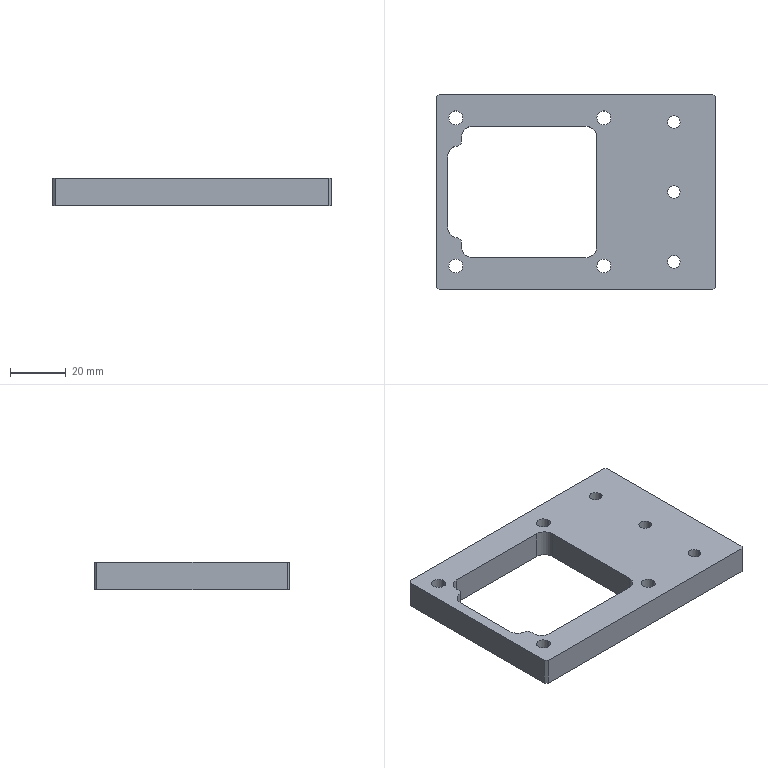Part | STEP file | MYT-A01-P13 | 1 solid | 47 faces | box 100 x 70 x 10 mm | volume 43994 mm3 | cylinder 26 | plane 21 | commonest cylinder face diameters 8 x12 5 x8 4.5 x6
STEP:
#1=CARTESIAN_POINT('',(39.,-25.,4.6));
#2=VERTEX_POINT('',#1);
#3=CARTESIAN_POINT('',(31.,-25.,4.6));
#4=VERTEX_POINT('',#3);
#5=CARTESIAN_POINT('',(35.,-25.,4.6));
#6=DIRECTION('',(0.,0.,-1.));
#7=DIRECTION('',(-1.,0.,0.));
#8=AXIS2_PLACEMENT_3D('',#5,#6,#7);
#9=CIRCLE('',#8,4.);
#10=EDGE_CURVE('',#2,#4,#9,.T.);
#11=ORIENTED_EDGE('',*,*,#10,.F.);
#12=CARTESIAN_POINT('',(39.,-25.,0.));
#13=VERTEX_POINT('',#12);
#14=CARTESIAN_POINT('',(39.,-25.,0.));
#15=DIRECTION('',(0.,0.,-1.));
#16=VECTOR('',#15,1000.);
#17=LINE('',#14,#16);
#18=EDGE_CURVE('',#2,#13,#17,.T.);
#19=ORIENTED_EDGE('',*,*,#18,.T.);
#20=CARTESIAN_POINT('',(31.,-25.,0.));
#21=VERTEX_POINT('',#20);
#22=CARTESIAN_POINT('',(35.,-25.,0.));
#23=DIRECTION('',(0.,0.,-1.));
#24=DIRECTION('',(-1.,0.,0.));
#25=AXIS2_PLACEMENT_3D('',#22,#23,#24);
#26=CIRCLE('',#25,4.);
#27=EDGE_CURVE('',#13,#21,#26,.T.);
#28=ORIENTED_EDGE('',*,*,#27,.T.);
#29=CARTESIAN_POINT('',(31.,-25.,0.));
#30=DIRECTION('',(0.,0.,-1.));
#31=VECTOR('',#30,1000.);
#32=LINE('',#29,#31);
#33=EDGE_CURVE('',#4,#21,#32,.T.);
#34=ORIENTED_EDGE('',*,*,#33,.F.);
#35=EDGE_LOOP('',(#11,#19,#28,#34));
#36=FACE_OUTER_BOUND('',#35,.T.);
#37=CARTESIAN_POINT('',(35.,-25.,0.));
#38=DIRECTION('',(0.,0.,-1.));
#39=DIRECTION('',(-1.,0.,0.));
#40=AXIS2_PLACEMENT_3D('',#37,#38,#39);
#41=CYLINDRICAL_SURFACE('',#40,4.);
#42=ADVANCED_FACE('',(#36),#41,.F.);
#43=CARTESIAN_POINT('',(37.25,-25.,10.));
#44=VERTEX_POINT('',#43);
#45=CARTESIAN_POINT('',(32.75,-25.,10.));
#46=VERTEX_POINT('',#45);
#47=CARTESIAN_POINT('',(35.,-25.,10.));
#48=DIRECTION('',(0.,0.,-1.));
#49=DIRECTION('',(-1.,0.,0.));
#50=AXIS2_PLACEMENT_3D('',#47,#48,#49);
#51=CIRCLE('',#50,2.25);
#52=EDGE_CURVE('',#44,#46,#51,.T.);
#53=ORIENTED_EDGE('',*,*,#52,.F.);
#54=CARTESIAN_POINT('',(37.25,-25.,4.6));
#55=VERTEX_POINT('',#54);
#56=CARTESIAN_POINT('',(37.25,-25.,0.));
#57=DIRECTION('',(0.,0.,-1.));
#58=VECTOR('',#57,1000.);
#59=LINE('',#56,#58);
#60=EDGE_CURVE('',#44,#55,#59,.T.);
#61=ORIENTED_EDGE('',*,*,#60,.T.);
#62=CARTESIAN_POINT('',(32.75,-25.,4.6));
#63=VERTEX_POINT('',#62);
#64=CARTESIAN_POINT('',(35.,-25.,4.6));
#65=DIRECTION('',(0.,0.,-1.));
#66=DIRECTION('',(-1.,0.,0.));
#67=AXIS2_PLACEMENT_3D('',#64,#65,#66);
#68=CIRCLE('',#67,2.25);
#69=EDGE_CURVE('',#55,#63,#68,.T.);
#70=ORIENTED_EDGE('',*,*,#69,.T.);
#71=CARTESIAN_POINT('',(32.75,-25.,0.));
#72=DIRECTION('',(0.,0.,-1.));
#73=VECTOR('',#72,1000.);
#74=LINE('',#71,#73);
#75=EDGE_CURVE('',#46,#63,#74,.T.);
#76=ORIENTED_EDGE('',*,*,#75,.F.);
#77=EDGE_LOOP('',(#53,#61,#70,#76));
#78=FACE_OUTER_BOUND('',#77,.T.);
#79=CARTESIAN_POINT('',(35.,-25.,0.));
#80=DIRECTION('',(0.,0.,-1.));
#81=DIRECTION('',(-1.,0.,0.));
#82=AXIS2_PLACEMENT_3D('',#79,#80,#81);
#83=CYLINDRICAL_SURFACE('',#82,2.25);
#84=ADVANCED_FACE('',(#78),#83,.F.);
#85=CARTESIAN_POINT('',(39.,0.,4.6));
#86=VERTEX_POINT('',#85);
#87=CARTESIAN_POINT('',(31.,0.,4.6));
#88=VERTEX_POINT('',#87);
#89=CARTESIAN_POINT('',(35.,0.,4.6));
#90=DIRECTION('',(0.,0.,-1.));
#91=DIRECTION('',(-1.,0.,0.));
#92=AXIS2_PLACEMENT_3D('',#89,#90,#91);
#93=CIRCLE('',#92,4.);
#94=EDGE_CURVE('',#86,#88,#93,.T.);
#95=ORIENTED_EDGE('',*,*,#94,.F.);
#96=CARTESIAN_POINT('',(39.,0.,0.));
#97=VERTEX_POINT('',#96);
#98=CARTESIAN_POINT('',(39.,0.,0.));
#99=DIRECTION('',(0.,0.,-1.));
#100=VECTOR('',#99,1000.);
#101=LINE('',#98,#100);
#102=EDGE_CURVE('',#86,#97,#101,.T.);
#103=ORIENTED_EDGE('',*,*,#102,.T.);
#104=CARTESIAN_POINT('',(31.,0.,0.));
#105=VERTEX_POINT('',#104);
#106=CARTESIAN_POINT('',(35.,0.,0.));
#107=DIRECTION('',(0.,0.,-1.));
#108=DIRECTION('',(-1.,0.,0.));
#109=AXIS2_PLACEMENT_3D('',#106,#107,#108);
#110=CIRCLE('',#109,4.);
#111=EDGE_CURVE('',#97,#105,#110,.T.);
#112=ORIENTED_EDGE('',*,*,#111,.T.);
#113=CARTESIAN_POINT('',(31.,0.,0.));
#114=DIRECTION('',(0.,0.,-1.));
#115=VECTOR('',#114,1000.);
#116=LINE('',#113,#115);
#117=EDGE_CURVE('',#88,#105,#116,.T.);
#118=ORIENTED_EDGE('',*,*,#117,.F.);
#119=EDGE_LOOP('',(#95,#103,#112,#118));
#120=FACE_OUTER_BOUND('',#119,.T.);
#121=CARTESIAN_POINT('',(35.,0.,0.));
#122=DIRECTION('',(0.,0.,-1.));
#123=DIRECTION('',(-1.,0.,0.));
#124=AXIS2_PLACEMENT_3D('',#121,#122,#123);
#125=CYLINDRICAL_SURFACE('',#124,4.);
#126=ADVANCED_FACE('',(#120),#125,.F.);
#127=CARTESIAN_POINT('',(37.25,0.,10.));
#128=VERTEX_POINT('',#127);
#129=CARTESIAN_POINT('',(32.75,0.,10.));
#130=VERTEX_POINT('',#129);
#131=CARTESIAN_POINT('',(35.,0.,10.));
#132=DIRECTION('',(0.,0.,-1.));
#133=DIRECTION('',(-1.,0.,0.));
#134=AXIS2_PLACEMENT_3D('',#131,#132,#133);
#135=CIRCLE('',#134,2.25);
#136=EDGE_CURVE('',#128,#130,#135,.T.);
#137=ORIENTED_EDGE('',*,*,#136,.F.);
#138=CARTESIAN_POINT('',(37.25,0.,4.6));
#139=VERTEX_POINT('',#138);
#140=CARTESIAN_POINT('',(37.25,0.,0.));
#141=DIRECTION('',(0.,0.,-1.));
#142=VECTOR('',#141,1000.);
#143=LINE('',#140,#142);
#144=EDGE_CURVE('',#128,#139,#143,.T.);
#145=ORIENTED_EDGE('',*,*,#144,.T.);
#146=CARTESIAN_POINT('',(32.75,0.,4.6));
#147=VERTEX_POINT('',#146);
#148=CARTESIAN_POINT('',(35.,0.,4.6));
#149=DIRECTION('',(0.,0.,-1.));
#150=DIRECTION('',(-1.,0.,0.));
#151=AXIS2_PLACEMENT_3D('',#148,#149,#150);
#152=CIRCLE('',#151,2.25);
#153=EDGE_CURVE('',#139,#147,#152,.T.);
#154=ORIENTED_EDGE('',*,*,#153,.T.);
#155=CARTESIAN_POINT('',(32.75,0.,0.));
#156=DIRECTION('',(0.,0.,-1.));
#157=VECTOR('',#156,1000.);
#158=LINE('',#155,#157);
#159=EDGE_CURVE('',#130,#147,#158,.T.);
#160=ORIENTED_EDGE('',*,*,#159,.F.);
#161=EDGE_LOOP('',(#137,#145,#154,#160));
#162=FACE_OUTER_BOUND('',#161,.T.);
#163=CARTESIAN_POINT('',(35.,0.,0.));
#164=DIRECTION('',(0.,0.,-1.));
#165=DIRECTION('',(-1.,0.,0.));
#166=AXIS2_PLACEMENT_3D('',#163,#164,#165);
#167=CYLINDRICAL_SURFACE('',#166,2.25);
#168=ADVANCED_FACE('',(#162),#167,.F.);
#169=CARTESIAN_POINT('',(39.,25.,4.6));
#170=VERTEX_POINT('',#169);
#171=CARTESIAN_POINT('',(31.,25.,4.6));
#172=VERTEX_POINT('',#171);
#173=CARTESIAN_POINT('',(35.,25.,4.6));
#174=DIRECTION('',(0.,0.,-1.));
#175=DIRECTION('',(-1.,0.,0.));
#176=AXIS2_PLACEMENT_3D('',#173,#174,#175);
#177=CIRCLE('',#176,4.);
#178=EDGE_CURVE('',#170,#172,#177,.T.);
#179=ORIENTED_EDGE('',*,*,#178,.F.);
#180=CARTESIAN_POINT('',(39.,25.,0.));
#181=VERTEX_POINT('',#180);
#182=CARTESIAN_POINT('',(39.,25.,0.));
#183=DIRECTION('',(0.,0.,-1.));
#184=VECTOR('',#183,1000.);
#185=LINE('',#182,#184);
#186=EDGE_CURVE('',#170,#181,#185,.T.);
#187=ORIENTED_EDGE('',*,*,#186,.T.);
#188=CARTESIAN_POINT('',(31.,25.,0.));
#189=VERTEX_POINT('',#188);
#190=CARTESIAN_POINT('',(35.,25.,0.));
#191=DIRECTION('',(0.,0.,-1.));
#192=DIRECTION('',(-1.,0.,0.));
#193=AXIS2_PLACEMENT_3D('',#190,#191,#192);
#194=CIRCLE('',#193,4.);
#195=EDGE_CURVE('',#181,#189,#194,.T.);
#196=ORIENTED_EDGE('',*,*,#195,.T.);
#197=CARTESIAN_POINT('',(31.,25.,0.));
#198=DIRECTION('',(0.,0.,-1.));
#199=VECTOR('',#198,1000.);
#200=LINE('',#197,#199);
#201=EDGE_CURVE('',#172,#189,#200,.T.);
#202=ORIENTED_EDGE('',*,*,#201,.F.);
#203=EDGE_LOOP('',(#179,#187,#196,#202));
#204=FACE_OUTER_BOUND('',#203,.T.);
#205=CARTESIAN_POINT('',(35.,25.,0.));
#206=DIRECTION('',(0.,0.,-1.));
#207=DIRECTION('',(-1.,0.,0.));
#208=AXIS2_PLACEMENT_3D('',#205,#206,#207);
#209=CYLINDRICAL_SURFACE('',#208,4.);
#210=ADVANCED_FACE('',(#204),#209,.F.);
#211=CARTESIAN_POINT('',(37.25,25.,10.));
#212=VERTEX_POINT('',#211);
#213=CARTESIAN_POINT('',(32.75,25.,10.));
#214=VERTEX_POINT('',#213);
#215=CARTESIAN_POINT('',(35.,25.,10.));
#216=DIRECTION('',(0.,0.,-1.));
#217=DIRECTION('',(-1.,0.,0.));
#218=AXIS2_PLACEMENT_3D('',#215,#216,#217);
#219=CIRCLE('',#218,2.25);
#220=EDGE_CURVE('',#212,#214,#219,.T.);
#221=ORIENTED_EDGE('',*,*,#220,.F.);
#222=CARTESIAN_POINT('',(37.25,25.,4.6));
#223=VERTEX_POINT('',#222);
#224=CARTESIAN_POINT('',(37.25,25.,0.));
#225=DIRECTION('',(0.,0.,-1.));
#226=VECTOR('',#225,1000.);
#227=LINE('',#224,#226);
#228=EDGE_CURVE('',#212,#223,#227,.T.);
#229=ORIENTED_EDGE('',*,*,#228,.T.);
#230=CARTESIAN_POINT('',(32.75,25.,4.6));
#231=VERTEX_POINT('',#230);
#232=CARTESIAN_POINT('',(35.,25.,4.6));
#233=DIRECTION('',(0.,0.,-1.));
#234=DIRECTION('',(-1.,0.,0.));
#235=AXIS2_PLACEMENT_3D('',#232,#233,#234);
#236=CIRCLE('',#235,2.25);
#237=EDGE_CURVE('',#223,#231,#236,.T.);
#238=ORIENTED_EDGE('',*,*,#237,.T.);
#239=CARTESIAN_POINT('',(32.75,25.,0.));
#240=DIRECTION('',(0.,0.,-1.));
#241=VECTOR('',#240,1000.);
#242=LINE('',#239,#241);
#243=EDGE_CURVE('',#214,#231,#242,.T.);
#244=ORIENTED_EDGE('',*,*,#243,.F.);
#245=EDGE_LOOP('',(#221,#229,#238,#244));
#246=FACE_OUTER_BOUND('',#245,.T.);
#247=CARTESIAN_POINT('',(35.,25.,0.));
#248=DIRECTION('',(0.,0.,-1.));
#249=DIRECTION('',(-1.,0.,0.));
#250=AXIS2_PLACEMENT_3D('',#247,#248,#249);
#251=CYLINDRICAL_SURFACE('',#250,2.25);
#252=ADVANCED_FACE('',(#246),#251,.F.);
#253=CARTESIAN_POINT('',(-45.5,26.5,0.));
#254=VERTEX_POINT('',#253);
#255=CARTESIAN_POINT('',(-40.5,26.5,0.));
#256=VERTEX_POINT('',#255);
#257=CARTESIAN_POINT('',(-43.,26.5,0.));
#258=DIRECTION('',(0.,0.,1.));
#259=DIRECTION('',(1.,0.,0.));
#260=AXIS2_PLACEMENT_3D('',#257,#258,#259);
#261=CIRCLE('',#260,2.5);
#262=EDGE_CURVE('',#254,#256,#261,.T.);
#263=ORIENTED_EDGE('',*,*,#262,.F.);
#264=CARTESIAN_POINT('',(-45.5,26.5,10.));
#265=VERTEX_POINT('',#264);
#266=CARTESIAN_POINT('',(-45.5,26.5,10.));
#267=DIRECTION('',(0.,0.,1.));
#268=VECTOR('',#267,1000.);
#269=LINE('',#266,#268);
#270=EDGE_CURVE('',#254,#265,#269,.T.);
#271=ORIENTED_EDGE('',*,*,#270,.T.);
#272=CARTESIAN_POINT('',(-40.5,26.5,10.));
#273=VERTEX_POINT('',#272);
#274=CARTESIAN_POINT('',(-43.,26.5,10.));
#275=DIRECTION('',(0.,0.,1.));
#276=DIRECTION('',(1.,0.,0.));
#277=AXIS2_PLACEMENT_3D('',#274,#275,#276);
#278=CIRCLE('',#277,2.5);
#279=EDGE_CURVE('',#265,#273,#278,.T.);
#280=ORIENTED_EDGE('',*,*,#279,.T.);
#281=CARTESIAN_POINT('',(-40.5,26.5,10.));
#282=DIRECTION('',(0.,0.,1.));
#283=VECTOR('',#282,1000.);
#284=LINE('',#281,#283);
#285=EDGE_CURVE('',#256,#273,#284,.T.);
#286=ORIENTED_EDGE('',*,*,#285,.F.);
#287=EDGE_LOOP('',(#263,#271,#280,#286));
#288=FACE_OUTER_BOUND('',#287,.T.);
#289=CARTESIAN_POINT('',(-43.,26.5,10.));
#290=DIRECTION('',(0.,0.,1.));
#291=DIRECTION('',(1.,0.,0.));
#292=AXIS2_PLACEMENT_3D('',#289,#290,#291);
#293=CYLINDRICAL_SURFACE('',#292,2.5);
#294=ADVANCED_FACE('',(#288),#293,.F.);
#295=CARTESIAN_POINT('',(-45.5,-26.5,0.));
#296=VERTEX_POINT('',#295);
#297=CARTESIAN_POINT('',(-40.5,-26.5,0.));
#298=VERTEX_POINT('',#297);
#299=CARTESIAN_POINT('',(-43.,-26.5,0.));
#300=DIRECTION('',(0.,0.,1.));
#301=DIRECTION('',(1.,0.,0.));
#302=AXIS2_PLACEMENT_3D('',#299,#300,#301);
#303=CIRCLE('',#302,2.5);
#304=EDGE_CURVE('',#296,#298,#303,.T.);
#305=ORIENTED_EDGE('',*,*,#304,.F.);
#306=CARTESIAN_POINT('',(-45.5,-26.5,10.));
#307=VERTEX_POINT('',#306);
#308=CARTESIAN_POINT('',(-45.5,-26.5,10.));
#309=DIRECTION('',(0.,0.,1.));
#310=VECTOR('',#309,1000.);
#311=LINE('',#308,#310);
#312=EDGE_CURVE('',#296,#307,#311,.T.);
#313=ORIENTED_EDGE('',*,*,#312,.T.);
#314=CARTESIAN_POINT('',(-40.5,-26.5,10.));
#315=VERTEX_POINT('',#314);
#316=CARTESIAN_POINT('',(-43.,-26.5,10.));
#317=DIRECTION('',(0.,0.,1.));
#318=DIRECTION('',(1.,0.,0.));
#319=AXIS2_PLACEMENT_3D('',#316,#317,#318);
#320=CIRCLE('',#319,2.5);
#321=EDGE_CURVE('',#307,#315,#320,.T.);
#322=ORIENTED_EDGE('',*,*,#321,.T.);
#323=CARTESIAN_POINT('',(-40.5,-26.5,10.));
#324=DIRECTION('',(0.,0.,1.));
#325=VECTOR('',#324,1000.);
#326=LINE('',#323,#325);
#327=EDGE_CURVE('',#298,#315,#326,.T.);
#328=ORIENTED_EDGE('',*,*,#327,.F.);
#329=EDGE_LOOP('',(#305,#313,#322,#328));
#330=FACE_OUTER_BOUND('',#329,.T.);
#331=CARTESIAN_POINT('',(-43.,-26.5,10.));
#332=DIRECTION('',(0.,0.,1.));
#333=DIRECTION('',(1.,0.,0.));
#334=AXIS2_PLACEMENT_3D('',#331,#332,#333);
#335=CYLINDRICAL_SURFACE('',#334,2.5);
#336=ADVANCED_FACE('',(#330),#335,.F.);
#337=CARTESIAN_POINT('',(7.5,-26.5,0.));
#338=VERTEX_POINT('',#337);
#339=CARTESIAN_POINT('',(12.5,-26.5,0.));
#340=VERTEX_POINT('',#339);
#341=CARTESIAN_POINT('',(10.,-26.5,0.));
#342=DIRECTION('',(0.,0.,1.));
#343=DIRECTION('',(1.,0.,0.));
#344=AXIS2_PLACEMENT_3D('',#341,#342,#343);
#345=CIRCLE('',#344,2.5);
#346=EDGE_CURVE('',#338,#340,#345,.T.);
#347=ORIENTED_EDGE('',*,*,#346,.F.);
#348=CARTESIAN_POINT('',(7.5,-26.5,10.));
#349=VERTEX_POINT('',#348);
#350=CARTESIAN_POINT('',(7.5,-26.5,10.));
#351=DIRECTION('',(0.,0.,1.));
#352=VECTOR('',#351,1000.);
#353=LINE('',#350,#352);
#354=EDGE_CURVE('',#338,#349,#353,.T.);
#355=ORIENTED_EDGE('',*,*,#354,.T.);
#356=CARTESIAN_POINT('',(12.5,-26.5,10.));
#357=VERTEX_POINT('',#356);
#358=CARTESIAN_POINT('',(10.,-26.5,10.));
#359=DIRECTION('',(0.,0.,1.));
#360=DIRECTION('',(1.,0.,0.));
#361=AXIS2_PLACEMENT_3D('',#358,#359,#360);
#362=CIRCLE('',#361,2.5);
#363=EDGE_CURVE('',#349,#357,#362,.T.);
#364=ORIENTED_EDGE('',*,*,#363,.T.);
#365=CARTESIAN_POINT('',(12.5,-26.5,10.));
#366=DIRECTION('',(0.,0.,1.));
#367=VECTOR('',#366,1000.);
#368=LINE('',#365,#367);
#369=EDGE_CURVE('',#340,#357,#368,.T.);
#370=ORIENTED_EDGE('',*,*,#369,.F.);
#371=EDGE_LOOP('',(#347,#355,#364,#370));
#372=FACE_OUTER_BOUND('',#371,.T.);
#373=CARTESIAN_POINT('',(10.,-26.5,10.));
#374=DIRECTION('',(0.,0.,1.));
#375=DIRECTION('',(1.,0.,0.));
#376=AXIS2_PLACEMENT_3D('',#373,#374,#375);
#377=CYLINDRICAL_SURFACE('',#376,2.5);
#378=ADVANCED_FACE('',(#372),#377,.F.);
#379=CARTESIAN_POINT('',(7.5,26.5,0.));
#380=VERTEX_POINT('',#379);
#381=CARTESIAN_POINT('',(12.5,26.5,0.));
#382=VERTEX_POINT('',#381);
#383=CARTESIAN_POINT('',(10.,26.5,0.));
#384=DIRECTION('',(0.,0.,1.));
#385=DIRECTION('',(1.,0.,0.));
#386=AXIS2_PLACEMENT_3D('',#383,#384,#385);
#387=CIRCLE('',#386,2.5);
#388=EDGE_CURVE('',#380,#382,#387,.T.);
#389=ORIENTED_EDGE('',*,*,#388,.F.);
#390=CARTESIAN_POINT('',(7.5,26.5,10.));
#391=VERTEX_POINT('',#390);
#392=CARTESIAN_POINT('',(7.5,26.5,10.));
#393=DIRECTION('',(0.,0.,1.));
#394=VECTOR('',#393,1000.);
#395=LINE('',#392,#394);
#396=EDGE_CURVE('',#380,#391,#395,.T.);
#397=ORIENTED_EDGE('',*,*,#396,.T.);
#398=CARTESIAN_POINT('',(12.5,26.5,10.));
#399=VERTEX_POINT('',#398);
#400=CARTESIAN_POINT('',(10.,26.5,10.));
#401=DIRECTION('',(0.,0.,1.));
#402=DIRECTION('',(1.,0.,0.));
#403=AXIS2_PLACEMENT_3D('',#400,#401,#402);
#404=CIRCLE('',#403,2.5);
#405=EDGE_CURVE('',#391,#399,#404,.T.);
#406=ORIENTED_EDGE('',*,*,#405,.T.);
#407=CARTESIAN_POINT('',(12.5,26.5,10.));
#408=DIRECTION('',(0.,0.,1.));
#409=VECTOR('',#408,1000.);
#410=LINE('',#407,#409);
#411=EDGE_CURVE('',#382,#399,#410,.T.);
#412=ORIENTED_EDGE('',*,*,#411,.F.);
#413=EDGE_LOOP('',(#389,#397,#406,#412));
#414=FACE_OUTER_BOUND('',#413,.T.);
#415=CARTESIAN_POINT('',(10.,26.5,10.));
#416=DIRECTION('',(0.,0.,1.));
#417=DIRECTION('',(1.,0.,0.));
#418=AXIS2_PLACEMENT_3D('',#415,#416,#417);
#419=CYLINDRICAL_SURFACE('',#418,2.5);
#420=ADVANCED_FACE('',(#414),#419,.F.);
#421=CARTESIAN_POINT('',(50.,-34.,0.));
#422=VERTEX_POINT('',#421);
#423=CARTESIAN_POINT('',(50.,34.,0.));
#424=VERTEX_POINT('',#423);
#425=CARTESIAN_POINT('',(50.,-35.,0.));
#426=DIRECTION('',(0.,1.,0.));
#427=VECTOR('',#426,1000.);
#428=LINE('',#425,#427);
#429=EDGE_CURVE('',#422,#424,#428,.T.);
#430=ORIENTED_EDGE('',*,*,#429,.T.);
#431=CARTESIAN_POINT('',(50.,34.,10.));
#432=VERTEX_POINT('',#431);
#433=CARTESIAN_POINT('',(50.,34.,10.));
#434=DIRECTION('',(0.,0.,1.));
#435=VECTOR('',#434,1000.);
#436=LINE('',#433,#435);
#437=EDGE_CURVE('',#424,#432,#436,.T.);
#438=ORIENTED_EDGE('',*,*,#437,.T.);
#439=CARTESIAN_POINT('',(50.,-34.,10.));
#440=VERTEX_POINT('',#439);
#441=CARTESIAN_POINT('',(50.,-35.,10.));
#442=DIRECTION('',(0.,1.,0.));
#443=VECTOR('',#442,1000.);
#444=LINE('',#441,#443);
#445=EDGE_CURVE('',#440,#432,#444,.T.);
#446=ORIENTED_EDGE('',*,*,#445,.F.);
#447=CARTESIAN_POINT('',(50.,-34.,10.));
#448=DIRECTION('',(0.,0.,-1.));
#449=VECTOR('',#448,1000.);
#450=LINE('',#447,#449);
#451=EDGE_CURVE('',#440,#422,#450,.T.);
#452=ORIENTED_EDGE('',*,*,#451,.T.);
#453=EDGE_LOOP('',(#430,#438,#446,#452));
#454=FACE_OUTER_BOUND('',#453,.T.);
#455=CARTESIAN_POINT('',(50.,-35.,10.));
#456=DIRECTION('',(-1.,0.,0.));
#457=DIRECTION('',(0.,0.,1.));
#458=AXIS2_PLACEMENT_3D('',#455,#456,#457);
#459=PLANE('',#458);
#460=ADVANCED_FACE('',(#454),#459,.F.);
#461=CARTESIAN_POINT('',(49.,35.,10.));
#462=VERTEX_POINT('',#461);
#463=CARTESIAN_POINT('',(-49.,35.,10.));
#464=VERTEX_POINT('',#463);
#465=CARTESIAN_POINT('',(-50.,35.,10.));
#466=DIRECTION('',(-1.,0.,0.));
#467=VECTOR('',#466,1000.);
#468=LINE('',#465,#467);
#469=EDGE_CURVE('',#462,#464,#468,.T.);
#470=ORIENTED_EDGE('',*,*,#469,.F.);
#471=CARTESIAN_POINT('',(49.,35.,0.));
#472=VERTEX_POINT('',#471);
#473=CARTESIAN_POINT('',(49.,35.,10.));
#474=DIRECTION('',(0.,0.,-1.));
#475=VECTOR('',#474,1000.);
#476=LINE('',#473,#475);
#477=EDGE_CURVE('',#462,#472,#476,.T.);
#478=ORIENTED_EDGE('',*,*,#477,.T.);
#479=CARTESIAN_POINT('',(-49.,35.,0.));
#480=VERTEX_POINT('',#479);
#481=CARTESIAN_POINT('',(-50.,35.,0.));
#482=DIRECTION('',(-1.,0.,0.));
#483=VECTOR('',#482,1000.);
#484=LINE('',#481,#483);
#485=EDGE_CURVE('',#472,#480,#484,.T.);
#486=ORIENTED_EDGE('',*,*,#485,.T.);
#487=CARTESIAN_POINT('',(-49.,35.,10.));
#488=DIRECTION('',(0.,0.,1.));
#489=VECTOR('',#488,1000.);
#490=LINE('',#487,#489);
#491=EDGE_CURVE('',#480,#464,#490,.T.);
#492=ORIENTED_EDGE('',*,*,#491,.T.);
#493=EDGE_LOOP('',(#470,#478,#486,#492));
#494=FACE_OUTER_BOUND('',#493,.T.);
#495=CARTESIAN_POINT('',(-50.,35.,10.));
#496=DIRECTION('',(0.,-1.,0.));
#497=DIRECTION('',(0.,0.,-1.));
#498=AXIS2_PLACEMENT_3D('',#495,#496,#497);
#499=PLANE('',#498);
#500=ADVANCED_FACE('',(#494),#499,.F.);
#501=CARTESIAN_POINT('',(-50.,34.,0.));
#502=VERTEX_POINT('',#501);
#503=CARTESIAN_POINT('',(-50.,-34.,0.));
#504=VERTEX_POINT('',#503);
#505=CARTESIAN_POINT('',(-50.,-35.,0.));
#506=DIRECTION('',(0.,-1.,0.));
#507=VECTOR('',#506,1000.);
#508=LINE('',#505,#507);
#509=EDGE_CURVE('',#502,#504,#508,.T.);
#510=ORIENTED_EDGE('',*,*,#509,.T.);
#511=CARTESIAN_POINT('',(-50.,-34.,10.));
#512=VERTEX_POINT('',#511);
#513=CARTESIAN_POINT('',(-50.,-34.,10.));
#514=DIRECTION('',(0.,0.,1.));
#515=VECTOR('',#514,1000.);
#516=LINE('',#513,#515);
#517=EDGE_CURVE('',#504,#512,#516,.T.);
#518=ORIENTED_EDGE('',*,*,#517,.T.);
#519=CARTESIAN_POINT('',(-50.,34.,10.));
#520=VERTEX_POINT('',#519);
#521=CARTESIAN_POINT('',(-50.,-35.,10.));
#522=DIRECTION('',(0.,-1.,0.));
#523=VECTOR('',#522,1000.);
#524=LINE('',#521,#523);
#525=EDGE_CURVE('',#520,#512,#524,.T.);
#526=ORIENTED_EDGE('',*,*,#525,.F.);
#527=CARTESIAN_POINT('',(-50.,34.,10.));
#528=DIRECTION('',(0.,0.,-1.));
#529=VECTOR('',#528,1000.);
#530=LINE('',#527,#529);
#531=EDGE_CURVE('',#520,#502,#530,.T.);
#532=ORIENTED_EDGE('',*,*,#531,.T.);
#533=EDGE_LOOP('',(#510,#518,#526,#532));
#534=FACE_OUTER_BOUND('',#533,.T.);
#535=CARTESIAN_POINT('',(-50.,-35.,10.));
#536=DIRECTION('',(1.,0.,0.));
#537=DIRECTION('',(0.,0.,-1.));
#538=AXIS2_PLACEMENT_3D('',#535,#536,#537);
#539=PLANE('',#538);
#540=ADVANCED_FACE('',(#534),#539,.F.);
#541=CARTESIAN_POINT('',(-49.,-35.,0.));
#542=VERTEX_POINT('',#541);
#543=CARTESIAN_POINT('',(49.,-35.,0.));
#544=VERTEX_POINT('',#543);
#545=CARTESIAN_POINT('',(-50.,-35.,0.));
#546=DIRECTION('',(1.,0.,0.));
#547=VECTOR('',#546,1000.);
#548=LINE('',#545,#547);
#549=EDGE_CURVE('',#542,#544,#548,.T.);
#550=ORIENTED_EDGE('',*,*,#549,.T.);
#551=CARTESIAN_POINT('',(49.,-35.,10.));
#552=VERTEX_POINT('',#551);
#553=CARTESIAN_POINT('',(49.,-35.,10.));
#554=DIRECTION('',(0.,0.,1.));
#555=VECTOR('',#554,1000.);
#556=LINE('',#553,#555);
#557=EDGE_CURVE('',#544,#552,#556,.T.);
#558=ORIENTED_EDGE('',*,*,#557,.T.);
#559=CARTESIAN_POINT('',(-49.,-35.,10.));
#560=VERTEX_POINT('',#559);
#561=CARTESIAN_POINT('',(-50.,-35.,10.));
#562=DIRECTION('',(1.,0.,0.));
#563=VECTOR('',#562,1000.);
#564=LINE('',#561,#563);
#565=EDGE_CURVE('',#560,#552,#564,.T.);
#566=ORIENTED_EDGE('',*,*,#565,.F.);
#567=CARTESIAN_POINT('',(-49.,-35.,10.));
#568=DIRECTION('',(0.,0.,-1.));
#569=VECTOR('',#568,1000.);
#570=LINE('',#567,#569);
#571=EDGE_CURVE('',#560,#542,#570,.T.);
#572=ORIENTED_EDGE('',*,*,#571,.T.);
#573=EDGE_LOOP('',(#550,#558,#566,#572));
#574=FACE_OUTER_BOUND('',#573,.T.);
#575=CARTESIAN_POINT('',(-50.,-35.,10.));
#576=DIRECTION('',(0.,1.,0.));
#577=DIRECTION('',(0.,0.,1.));
#578=AXIS2_PLACEMENT_3D('',#575,#576,#577);
#579=PLANE('',#578);
#580=ADVANCED_FACE('',(#574),#579,.F.);
#581=CARTESIAN_POINT('',(35.,-25.,10.));
#582=DIRECTION('',(0.,0.,-1.));
#583=DIRECTION('',(-1.,0.,0.));
#584=AXIS2_PLACEMENT_3D('',#581,#582,#583);
#585=CIRCLE('',#584,2.25);
#586=EDGE_CURVE('',#46,#44,#585,.T.);
#587=ORIENTED_EDGE('',*,*,#586,.T.);
#588=ORIENTED_EDGE('',*,*,#52,.T.);
#589=EDGE_LOOP('',(#587,#588));
#590=FACE_BOUND('',#589,.T.);
#591=CARTESIAN_POINT('',(35.,0.,10.));
#592=DIRECTION('',(0.,0.,-1.));
#593=DIRECTION('',(-1.,0.,0.));
#594=AXIS2_PLACEMENT_3D('',#591,#592,#593);
#595=CIRCLE('',#594,2.25);
#596=EDGE_CURVE('',#130,#128,#595,.T.);
#597=ORIENTED_EDGE('',*,*,#596,.T.);
#598=ORIENTED_EDGE('',*,*,#136,.T.);
#599=EDGE_LOOP('',(#597,#598));
#600=FACE_BOUND('',#599,.T.);
#601=CARTESIAN_POINT('',(35.,25.,10.));
#602=DIRECTION('',(0.,0.,-1.));
#603=DIRECTION('',(-1.,0.,0.));
#604=AXIS2_PLACEMENT_3D('',#601,#602,#603);
#605=CIRCLE('',#604,2.25);
#606=EDGE_CURVE('',#214,#212,#605,.T.);
#607=ORIENTED_EDGE('',*,*,#606,.T.);
#608=ORIENTED_EDGE('',*,*,#220,.T.);
#609=EDGE_LOOP('',(#607,#608));
#610=FACE_BOUND('',#609,.T.);
#611=CARTESIAN_POINT('',(-41.,-19.5,10.));
#612=VERTEX_POINT('',#611);
#613=CARTESIAN_POINT('',(-41.,-17.5,10.));
#614=VERTEX_POINT('',#613);
#615=CARTESIAN_POINT('',(-41.,-23.5,10.));
#616=DIRECTION('',(0.,1.,0.));
#617=VECTOR('',#616,1000.);
#618=LINE('',#615,#617);
#619=EDGE_CURVE('',#612,#614,#618,.T.);
#620=ORIENTED_EDGE('',*,*,#619,.T.);
#621=CARTESIAN_POINT('',(-42.,-16.5,10.));
#622=VERTEX_POINT('',#621);
#623=CARTESIAN_POINT('',(-41.,-17.5,10.));
#624=DIRECTION('',(-0.7071,0.7071,0.));
#625=VECTOR('',#624,1000.);
#626=LINE('',#623,#625);
#627=EDGE_CURVE('',#614,#622,#626,.T.);
#628=ORIENTED_EDGE('',*,*,#627,.T.);
#629=CARTESIAN_POINT('',(-46.,-12.5,10.));
#630=VERTEX_POINT('',#629);
#631=CARTESIAN_POINT('',(-42.,-12.5,10.));
#632=DIRECTION('',(0.,0.,-1.));
#633=DIRECTION('',(-1.,0.,0.));
#634=AXIS2_PLACEMENT_3D('',#631,#632,#633);
#635=CIRCLE('',#634,4.);
#636=EDGE_CURVE('',#622,#630,#635,.T.);
#637=ORIENTED_EDGE('',*,*,#636,.T.);
#638=CARTESIAN_POINT('',(-46.,12.5,10.));
#639=VERTEX_POINT('',#638);
#640=CARTESIAN_POINT('',(-46.,23.5,10.));
#641=DIRECTION('',(0.,-1.,0.));
#642=VECTOR('',#641,1000.);
#643=LINE('',#640,#642);
#644=EDGE_CURVE('',#639,#630,#643,.T.);
#645=ORIENTED_EDGE('',*,*,#644,.F.);
#646=CARTESIAN_POINT('',(-42.,16.5,10.));
#647=VERTEX_POINT('',#646);
#648=CARTESIAN_POINT('',(-42.,12.5,10.));
#649=DIRECTION('',(0.,0.,-1.));
#650=DIRECTION('',(-1.,0.,0.));
#651=AXIS2_PLACEMENT_3D('',#648,#649,#650);
#652=CIRCLE('',#651,4.);
#653=EDGE_CURVE('',#639,#647,#652,.T.);
#654=ORIENTED_EDGE('',*,*,#653,.T.);
#655=CARTESIAN_POINT('',(-41.,17.5,10.));
#656=VERTEX_POINT('',#655);
#657=CARTESIAN_POINT('',(-42.,16.5,10.));
#658=DIRECTION('',(0.7071,0.7071,0.));
#659=VECTOR('',#658,1000.);
#660=LINE('',#657,#659);
#661=EDGE_CURVE('',#647,#656,#660,.T.);
#662=ORIENTED_EDGE('',*,*,#661,.T.);
#663=CARTESIAN_POINT('',(-41.,19.5,10.));
#664=VERTEX_POINT('',#663);
#665=CARTESIAN_POINT('',(-41.,23.5,10.));
#666=DIRECTION('',(0.,1.,0.));
#667=VECTOR('',#666,1000.);
#668=LINE('',#665,#667);
#669=EDGE_CURVE('',#656,#664,#668,.T.);
#670=ORIENTED_EDGE('',*,*,#669,.T.);
#671=CARTESIAN_POINT('',(-37.,23.5,10.));
#672=VERTEX_POINT('',#671);
#673=CARTESIAN_POINT('',(-37.,19.5,10.));
#674=DIRECTION('',(0.,0.,-1.));
#675=DIRECTION('',(-1.,0.,0.));
#676=AXIS2_PLACEMENT_3D('',#673,#674,#675);
#677=CIRCLE('',#676,4.);
#678=EDGE_CURVE('',#664,#672,#677,.T.);
#679=ORIENTED_EDGE('',*,*,#678,.T.);
#680=CARTESIAN_POINT('',(3.5,23.5,10.));
#681=VERTEX_POINT('',#680);
#682=CARTESIAN_POINT('',(-46.,23.5,10.));
#683=DIRECTION('',(-1.,0.,0.));
#684=VECTOR('',#683,1000.);
#685=LINE('',#682,#684);
#686=EDGE_CURVE('',#681,#672,#685,.T.);
#687=ORIENTED_EDGE('',*,*,#686,.F.);
#688=CARTESIAN_POINT('',(7.5,19.5,10.));
#689=VERTEX_POINT('',#688);
#690=CARTESIAN_POINT('',(3.5,19.5,10.));
#691=DIRECTION('',(0.,0.,-1.));
#692=DIRECTION('',(-1.,0.,0.));
#693=AXIS2_PLACEMENT_3D('',#690,#691,#692);
#694=CIRCLE('',#693,4.);
#695=EDGE_CURVE('',#681,#689,#694,.T.);
#696=ORIENTED_EDGE('',*,*,#695,.T.);
#697=CARTESIAN_POINT('',(7.5,-19.5,10.));
#698=VERTEX_POINT('',#697);
#699=CARTESIAN_POINT('',(7.5,23.5,10.));
#700=DIRECTION('',(0.,1.,0.));
#701=VECTOR('',#700,1000.);
#702=LINE('',#699,#701);
#703=EDGE_CURVE('',#698,#689,#702,.T.);
#704=ORIENTED_EDGE('',*,*,#703,.F.);
#705=CARTESIAN_POINT('',(3.5,-23.5,10.));
#706=VERTEX_POINT('',#705);
#707=CARTESIAN_POINT('',(3.5,-19.5,10.));
#708=DIRECTION('',(0.,0.,-1.));
#709=DIRECTION('',(-1.,0.,0.));
#710=AXIS2_PLACEMENT_3D('',#707,#708,#709);
#711=CIRCLE('',#710,4.);
#712=EDGE_CURVE('',#698,#706,#711,.T.);
#713=ORIENTED_EDGE('',*,*,#712,.T.);
#714=CARTESIAN_POINT('',(-37.,-23.5,10.));
#715=VERTEX_POINT('',#714);
#716=CARTESIAN_POINT('',(-46.,-23.5,10.));
#717=DIRECTION('',(1.,0.,0.));
#718=VECTOR('',#717,1000.);
#719=LINE('',#716,#718);
#720=EDGE_CURVE('',#715,#706,#719,.T.);
#721=ORIENTED_EDGE('',*,*,#720,.F.);
#722=CARTESIAN_POINT('',(-37.,-19.5,10.));
#723=DIRECTION('',(0.,0.,-1.));
#724=DIRECTION('',(-1.,0.,0.));
#725=AXIS2_PLACEMENT_3D('',#722,#723,#724);
#726=CIRCLE('',#725,4.);
#727=EDGE_CURVE('',#715,#612,#726,.T.);
#728=ORIENTED_EDGE('',*,*,#727,.T.);
#729=EDGE_LOOP('',(#620,#628,#637,#645,#654,#662,#670,#679,#687,#696,#704,#713,#721,#728));
#730=FACE_BOUND('',#729,.T.);
#731=CARTESIAN_POINT('',(-43.,26.5,10.));
#732=DIRECTION('',(0.,0.,1.));
#733=DIRECTION('',(1.,0.,0.));
#734=AXIS2_PLACEMENT_3D('',#731,#732,#733);
#735=CIRCLE('',#734,2.5);
#736=EDGE_CURVE('',#273,#265,#735,.T.);
#737=ORIENTED_EDGE('',*,*,#736,.F.);
#738=ORIENTED_EDGE('',*,*,#279,.F.);
#739=EDGE_LOOP('',(#737,#738));
#740=FACE_BOUND('',#739,.T.);
#741=CARTESIAN_POINT('',(-43.,-26.5,10.));
#742=DIRECTION('',(0.,0.,1.));
#743=DIRECTION('',(1.,0.,0.));
#744=AXIS2_PLACEMENT_3D('',#741,#742,#743);
#745=CIRCLE('',#744,2.5);
#746=EDGE_CURVE('',#315,#307,#745,.T.);
#747=ORIENTED_EDGE('',*,*,#746,.F.);
#748=ORIENTED_EDGE('',*,*,#321,.F.);
#749=EDGE_LOOP('',(#747,#748));
#750=FACE_BOUND('',#749,.T.);
#751=CARTESIAN_POINT('',(10.,-26.5,10.));
#752=DIRECTION('',(0.,0.,1.));
#753=DIRECTION('',(1.,0.,0.));
#754=AXIS2_PLACEMENT_3D('',#751,#752,#753);
#755=CIRCLE('',#754,2.5);
#756=EDGE_CURVE('',#357,#349,#755,.T.);
#757=ORIENTED_EDGE('',*,*,#756,.F.);
#758=ORIENTED_EDGE('',*,*,#363,.F.);
#759=EDGE_LOOP('',(#757,#758));
#760=FACE_BOUND('',#759,.T.);
#761=CARTESIAN_POINT('',(10.,26.5,10.));
#762=DIRECTION('',(0.,0.,1.));
#763=DIRECTION('',(1.,0.,0.));
#764=AXIS2_PLACEMENT_3D('',#761,#762,#763);
#765=CIRCLE('',#764,2.5);
#766=EDGE_CURVE('',#399,#391,#765,.T.);
#767=ORIENTED_EDGE('',*,*,#766,.F.);
#768=ORIENTED_EDGE('',*,*,#405,.F.);
#769=EDGE_LOOP('',(#767,#768));
#770=FACE_BOUND('',#769,.T.);
#771=ORIENTED_EDGE('',*,*,#445,.T.);
#772=CARTESIAN_POINT('',(49.,35.,10.));
#773=DIRECTION('',(-0.7071,0.7071,0.));
#774=VECTOR('',#773,1000.);
#775=LINE('',#772,#774);
#776=EDGE_CURVE('',#432,#462,#775,.T.);
#777=ORIENTED_EDGE('',*,*,#776,.T.);
#778=ORIENTED_EDGE('',*,*,#469,.T.);
#779=CARTESIAN_POINT('',(-50.,34.,10.));
#780=DIRECTION('',(-0.7071,-0.7071,0.));
#781=VECTOR('',#780,1000.);
#782=LINE('',#779,#781);
#783=EDGE_CURVE('',#464,#520,#782,.T.);
#784=ORIENTED_EDGE('',*,*,#783,.T.);
#785=ORIENTED_EDGE('',*,*,#525,.T.);
#786=CARTESIAN_POINT('',(-49.,-35.,10.));
#787=DIRECTION('',(0.7071,-0.7071,0.));
#788=VECTOR('',#787,1000.);
#789=LINE('',#786,#788);
#790=EDGE_CURVE('',#512,#560,#789,.T.);
#791=ORIENTED_EDGE('',*,*,#790,.T.);
#792=ORIENTED_EDGE('',*,*,#565,.T.);
#793=CARTESIAN_POINT('',(50.,-34.,10.));
#794=DIRECTION('',(0.7071,0.7071,0.));
#795=VECTOR('',#794,1000.);
#796=LINE('',#793,#795);
#797=EDGE_CURVE('',#552,#440,#796,.T.);
#798=ORIENTED_EDGE('',*,*,#797,.T.);
#799=EDGE_LOOP('',(#771,#777,#778,#784,#785,#791,#792,#798));
#800=FACE_OUTER_BOUND('',#799,.T.);
#801=CARTESIAN_POINT('',(0.,0.,10.));
#802=DIRECTION('',(0.,0.,-1.));
#803=DIRECTION('',(-1.,0.,0.));
#804=AXIS2_PLACEMENT_3D('',#801,#802,#803);
#805=PLANE('',#804);
#806=ADVANCED_FACE('',(#590,#600,#610,#730,#740,#750,#760,#770,#800),#805,.F.);
#807=CARTESIAN_POINT('',(35.,-25.,0.));
#808=DIRECTION('',(0.,0.,-1.));
#809=DIRECTION('',(-1.,0.,0.));
#810=AXIS2_PLACEMENT_3D('',#807,#808,#809);
#811=CIRCLE('',#810,4.);
#812=EDGE_CURVE('',#21,#13,#811,.T.);
#813=ORIENTED_EDGE('',*,*,#812,.F.);
#814=ORIENTED_EDGE('',*,*,#27,.F.);
#815=EDGE_LOOP('',(#813,#814));
#816=FACE_BOUND('',#815,.T.);
#817=CARTESIAN_POINT('',(35.,0.,0.));
#818=DIRECTION('',(0.,0.,-1.));
#819=DIRECTION('',(-1.,0.,0.));
#820=AXIS2_PLACEMENT_3D('',#817,#818,#819);
#821=CIRCLE('',#820,4.);
#822=EDGE_CURVE('',#105,#97,#821,.T.);
#823=ORIENTED_EDGE('',*,*,#822,.F.);
#824=ORIENTED_EDGE('',*,*,#111,.F.);
#825=EDGE_LOOP('',(#823,#824));
#826=FACE_BOUND('',#825,.T.);
#827=CARTESIAN_POINT('',(35.,25.,0.));
#828=DIRECTION('',(0.,0.,-1.));
#829=DIRECTION('',(-1.,0.,0.));
#830=AXIS2_PLACEMENT_3D('',#827,#828,#829);
#831=CIRCLE('',#830,4.);
#832=EDGE_CURVE('',#189,#181,#831,.T.);
#833=ORIENTED_EDGE('',*,*,#832,.F.);
#834=ORIENTED_EDGE('',*,*,#195,.F.);
#835=EDGE_LOOP('',(#833,#834));
#836=FACE_BOUND('',#835,.T.);
#837=CARTESIAN_POINT('',(-46.,-12.5,0.));
#838=VERTEX_POINT('',#837);
#839=CARTESIAN_POINT('',(-42.,-16.5,0.));
#840=VERTEX_POINT('',#839);
#841=CARTESIAN_POINT('',(-42.,-12.5,0.));
#842=DIRECTION('',(0.,0.,1.));
#843=DIRECTION('',(-1.,0.,0.));
#844=AXIS2_PLACEMENT_3D('',#841,#842,#843);
#845=CIRCLE('',#844,4.);
#846=EDGE_CURVE('',#838,#840,#845,.T.);
#847=ORIENTED_EDGE('',*,*,#846,.T.);
#848=CARTESIAN_POINT('',(-41.,-17.5,0.));
#849=VERTEX_POINT('',#848);
#850=CARTESIAN_POINT('',(-29.25,-29.25,0.));
#851=DIRECTION('',(0.7071,-0.7071,0.));
#852=VECTOR('',#851,1000.);
#853=LINE('',#850,#852);
#854=EDGE_CURVE('',#840,#849,#853,.T.);
#855=ORIENTED_EDGE('',*,*,#854,.T.);
#856=CARTESIAN_POINT('',(-41.,-19.5,0.));
#857=VERTEX_POINT('',#856);
#858=CARTESIAN_POINT('',(-41.,-23.5,0.));
#859=DIRECTION('',(0.,1.,0.));
#860=VECTOR('',#859,1000.);
#861=LINE('',#858,#860);
#862=EDGE_CURVE('',#857,#849,#861,.T.);
#863=ORIENTED_EDGE('',*,*,#862,.F.);
#864=CARTESIAN_POINT('',(-37.,-23.5,0.));
#865=VERTEX_POINT('',#864);
#866=CARTESIAN_POINT('',(-37.,-19.5,0.));
#867=DIRECTION('',(0.,0.,1.));
#868=DIRECTION('',(-1.,0.,0.));
#869=AXIS2_PLACEMENT_3D('',#866,#867,#868);
#870=CIRCLE('',#869,4.);
#871=EDGE_CURVE('',#857,#865,#870,.T.);
#872=ORIENTED_EDGE('',*,*,#871,.T.);
#873=CARTESIAN_POINT('',(3.5,-23.5,0.));
#874=VERTEX_POINT('',#873);
#875=CARTESIAN_POINT('',(-46.,-23.5,0.));
#876=DIRECTION('',(1.,0.,0.));
#877=VECTOR('',#876,1000.);
#878=LINE('',#875,#877);
#879=EDGE_CURVE('',#865,#874,#878,.T.);
#880=ORIENTED_EDGE('',*,*,#879,.T.);
#881=CARTESIAN_POINT('',(7.5,-19.5,0.));
#882=VERTEX_POINT('',#881);
#883=CARTESIAN_POINT('',(3.5,-19.5,0.));
#884=DIRECTION('',(0.,0.,1.));
#885=DIRECTION('',(-1.,0.,0.));
#886=AXIS2_PLACEMENT_3D('',#883,#884,#885);
#887=CIRCLE('',#886,4.);
#888=EDGE_CURVE('',#874,#882,#887,.T.);
#889=ORIENTED_EDGE('',*,*,#888,.T.);
#890=CARTESIAN_POINT('',(7.5,19.5,0.));
#891=VERTEX_POINT('',#890);
#892=CARTESIAN_POINT('',(7.5,23.5,0.));
#893=DIRECTION('',(0.,1.,0.));
#894=VECTOR('',#893,1000.);
#895=LINE('',#892,#894);
#896=EDGE_CURVE('',#882,#891,#895,.T.);
#897=ORIENTED_EDGE('',*,*,#896,.T.);
#898=CARTESIAN_POINT('',(3.5,23.5,0.));
#899=VERTEX_POINT('',#898);
#900=CARTESIAN_POINT('',(3.5,19.5,0.));
#901=DIRECTION('',(0.,0.,1.));
#902=DIRECTION('',(-1.,0.,0.));
#903=AXIS2_PLACEMENT_3D('',#900,#901,#902);
#904=CIRCLE('',#903,4.);
#905=EDGE_CURVE('',#891,#899,#904,.T.);
#906=ORIENTED_EDGE('',*,*,#905,.T.);
#907=CARTESIAN_POINT('',(-37.,23.5,0.));
#908=VERTEX_POINT('',#907);
#909=CARTESIAN_POINT('',(-46.,23.5,0.));
#910=DIRECTION('',(-1.,0.,0.));
#911=VECTOR('',#910,1000.);
#912=LINE('',#909,#911);
#913=EDGE_CURVE('',#899,#908,#912,.T.);
#914=ORIENTED_EDGE('',*,*,#913,.T.);
#915=CARTESIAN_POINT('',(-41.,19.5,0.));
#916=VERTEX_POINT('',#915);
#917=CARTESIAN_POINT('',(-37.,19.5,0.));
#918=DIRECTION('',(0.,0.,1.));
#919=DIRECTION('',(-1.,0.,0.));
#920=AXIS2_PLACEMENT_3D('',#917,#918,#919);
#921=CIRCLE('',#920,4.);
#922=EDGE_CURVE('',#908,#916,#921,.T.);
#923=ORIENTED_EDGE('',*,*,#922,.T.);
#924=CARTESIAN_POINT('',(-41.,17.5,0.));
#925=VERTEX_POINT('',#924);
#926=CARTESIAN_POINT('',(-41.,23.5,0.));
#927=DIRECTION('',(0.,1.,0.));
#928=VECTOR('',#927,1000.);
#929=LINE('',#926,#928);
#930=EDGE_CURVE('',#925,#916,#929,.T.);
#931=ORIENTED_EDGE('',*,*,#930,.F.);
#932=CARTESIAN_POINT('',(-42.,16.5,0.));
#933=VERTEX_POINT('',#932);
#934=CARTESIAN_POINT('',(-29.25,29.25,0.));
#935=DIRECTION('',(-0.7071,-0.7071,0.));
#936=VECTOR('',#935,1000.);
#937=LINE('',#934,#936);
#938=EDGE_CURVE('',#925,#933,#937,.T.);
#939=ORIENTED_EDGE('',*,*,#938,.T.);
#940=CARTESIAN_POINT('',(-46.,12.5,0.));
#941=VERTEX_POINT('',#940);
#942=CARTESIAN_POINT('',(-42.,12.5,0.));
#943=DIRECTION('',(0.,0.,1.));
#944=DIRECTION('',(-1.,0.,0.));
#945=AXIS2_PLACEMENT_3D('',#942,#943,#944);
#946=CIRCLE('',#945,4.);
#947=EDGE_CURVE('',#933,#941,#946,.T.);
#948=ORIENTED_EDGE('',*,*,#947,.T.);
#949=CARTESIAN_POINT('',(-46.,23.5,0.));
#950=DIRECTION('',(0.,-1.,0.));
#951=VECTOR('',#950,1000.);
#952=LINE('',#949,#951);
#953=EDGE_CURVE('',#941,#838,#952,.T.);
#954=ORIENTED_EDGE('',*,*,#953,.T.);
#955=EDGE_LOOP('',(#847,#855,#863,#872,#880,#889,#897,#906,#914,#923,#931,#939,#948,#954));
#956=FACE_BOUND('',#955,.T.);
#957=CARTESIAN_POINT('',(-43.,26.5,0.));
#958=DIRECTION('',(0.,0.,1.));
#959=DIRECTION('',(1.,0.,0.));
#960=AXIS2_PLACEMENT_3D('',#957,#958,#959);
#961=CIRCLE('',#960,2.5);
#962=EDGE_CURVE('',#256,#254,#961,.T.);
#963=ORIENTED_EDGE('',*,*,#962,.T.);
#964=ORIENTED_EDGE('',*,*,#262,.T.);
#965=EDGE_LOOP('',(#963,#964));
#966=FACE_BOUND('',#965,.T.);
#967=CARTESIAN_POINT('',(-43.,-26.5,0.));
#968=DIRECTION('',(0.,0.,1.));
#969=DIRECTION('',(1.,0.,0.));
#970=AXIS2_PLACEMENT_3D('',#967,#968,#969);
#971=CIRCLE('',#970,2.5);
#972=EDGE_CURVE('',#298,#296,#971,.T.);
#973=ORIENTED_EDGE('',*,*,#972,.T.);
#974=ORIENTED_EDGE('',*,*,#304,.T.);
#975=EDGE_LOOP('',(#973,#974));
#976=FACE_BOUND('',#975,.T.);
#977=CARTESIAN_POINT('',(10.,-26.5,0.));
#978=DIRECTION('',(0.,0.,1.));
#979=DIRECTION('',(1.,0.,0.));
#980=AXIS2_PLACEMENT_3D('',#977,#978,#979);
#981=CIRCLE('',#980,2.5);
#982=EDGE_CURVE('',#340,#338,#981,.T.);
#983=ORIENTED_EDGE('',*,*,#982,.T.);
#984=ORIENTED_EDGE('',*,*,#346,.T.);
#985=EDGE_LOOP('',(#983,#984));
#986=FACE_BOUND('',#985,.T.);
#987=CARTESIAN_POINT('',(10.,26.5,0.));
#988=DIRECTION('',(0.,0.,1.));
#989=DIRECTION('',(1.,0.,0.));
#990=AXIS2_PLACEMENT_3D('',#987,#988,#989);
#991=CIRCLE('',#990,2.5);
#992=EDGE_CURVE('',#382,#380,#991,.T.);
#993=ORIENTED_EDGE('',*,*,#992,.T.);
#994=ORIENTED_EDGE('',*,*,#388,.T.);
#995=EDGE_LOOP('',(#993,#994));
#996=FACE_BOUND('',#995,.T.);
#997=ORIENTED_EDGE('',*,*,#485,.F.);
#998=CARTESIAN_POINT('',(42.,42.,0.));
#999=DIRECTION('',(0.7071,-0.7071,0.));
#1000=VECTOR('',#999,1000.);
#1001=LINE('',#998,#1000);
#1002=EDGE_CURVE('',#472,#424,#1001,.T.);
#1003=ORIENTED_EDGE('',*,*,#1002,.T.);
#1004=ORIENTED_EDGE('',*,*,#429,.F.);
#1005=CARTESIAN_POINT('',(42.,-42.,0.));
#1006=DIRECTION('',(-0.7071,-0.7071,0.));
#1007=VECTOR('',#1006,1000.);
#1008=LINE('',#1005,#1007);
#1009=EDGE_CURVE('',#422,#544,#1008,.T.);
#1010=ORIENTED_EDGE('',*,*,#1009,.T.);
#1011=ORIENTED_EDGE('',*,*,#549,.F.);
#1012=CARTESIAN_POINT('',(-42.,-42.,0.));
#1013=DIRECTION('',(-0.7071,0.7071,0.));
#1014=VECTOR('',#1013,1000.);
#1015=LINE('',#1012,#1014);
#1016=EDGE_CURVE('',#542,#504,#1015,.T.);
#1017=ORIENTED_EDGE('',*,*,#1016,.T.);
#1018=ORIENTED_EDGE('',*,*,#509,.F.);
#1019=CARTESIAN_POINT('',(-42.,42.,0.));
#1020=DIRECTION('',(0.7071,0.7071,0.));
#1021=VECTOR('',#1020,1000.);
#1022=LINE('',#1019,#1021);
#1023=EDGE_CURVE('',#502,#480,#1022,.T.);
#1024=ORIENTED_EDGE('',*,*,#1023,.T.);
#1025=EDGE_LOOP('',(#997,#1003,#1004,#1010,#1011,#1017,#1018,#1024));
#1026=FACE_OUTER_BOUND('',#1025,.T.);
#1027=CARTESIAN_POINT('',(0.,0.,0.));
#1028=DIRECTION('',(0.,0.,-1.));
#1029=DIRECTION('',(-1.,0.,0.));
#1030=AXIS2_PLACEMENT_3D('',#1027,#1028,#1029);
#1031=PLANE('',#1030);
#1032=ADVANCED_FACE('',(#816,#826,#836,#956,#966,#976,#986,#996,#1026),#1031,.T.);
#1033=ORIENTED_EDGE('',*,*,#396,.F.);
#1034=ORIENTED_EDGE('',*,*,#992,.F.);
#1035=ORIENTED_EDGE('',*,*,#411,.T.);
#1036=ORIENTED_EDGE('',*,*,#766,.T.);
#1037=EDGE_LOOP('',(#1033,#1034,#1035,#1036));
#1038=FACE_OUTER_BOUND('',#1037,.T.);
#1039=CARTESIAN_POINT('',(10.,26.5,10.));
#1040=DIRECTION('',(0.,0.,1.));
#1041=DIRECTION('',(1.,0.,0.));
#1042=AXIS2_PLACEMENT_3D('',#1039,#1040,#1041);
#1043=CYLINDRICAL_SURFACE('',#1042,2.5);
#1044=ADVANCED_FACE('',(#1038),#1043,.F.);
#1045=ORIENTED_EDGE('',*,*,#354,.F.);
#1046=ORIENTED_EDGE('',*,*,#982,.F.);
#1047=ORIENTED_EDGE('',*,*,#369,.T.);
#1048=ORIENTED_EDGE('',*,*,#756,.T.);
#1049=EDGE_LOOP('',(#1045,#1046,#1047,#1048));
#1050=FACE_OUTER_BOUND('',#1049,.T.);
#1051=CARTESIAN_POINT('',(10.,-26.5,10.));
#1052=DIRECTION('',(0.,0.,1.));
#1053=DIRECTION('',(1.,0.,0.));
#1054=AXIS2_PLACEMENT_3D('',#1051,#1052,#1053);
#1055=CYLINDRICAL_SURFACE('',#1054,2.5);
#1056=ADVANCED_FACE('',(#1050),#1055,.F.);
#1057=ORIENTED_EDGE('',*,*,#312,.F.);
#1058=ORIENTED_EDGE('',*,*,#972,.F.);
#1059=ORIENTED_EDGE('',*,*,#327,.T.);
#1060=ORIENTED_EDGE('',*,*,#746,.T.);
#1061=EDGE_LOOP('',(#1057,#1058,#1059,#1060));
#1062=FACE_OUTER_BOUND('',#1061,.T.);
#1063=CARTESIAN_POINT('',(-43.,-26.5,10.));
#1064=DIRECTION('',(0.,0.,1.));
#1065=DIRECTION('',(1.,0.,0.));
#1066=AXIS2_PLACEMENT_3D('',#1063,#1064,#1065);
#1067=CYLINDRICAL_SURFACE('',#1066,2.5);
#1068=ADVANCED_FACE('',(#1062),#1067,.F.);
#1069=ORIENTED_EDGE('',*,*,#270,.F.);
#1070=ORIENTED_EDGE('',*,*,#962,.F.);
#1071=ORIENTED_EDGE('',*,*,#285,.T.);
#1072=ORIENTED_EDGE('',*,*,#736,.T.);
#1073=EDGE_LOOP('',(#1069,#1070,#1071,#1072));
#1074=FACE_OUTER_BOUND('',#1073,.T.);
#1075=CARTESIAN_POINT('',(-43.,26.5,10.));
#1076=DIRECTION('',(0.,0.,1.));
#1077=DIRECTION('',(1.,0.,0.));
#1078=AXIS2_PLACEMENT_3D('',#1075,#1076,#1077);
#1079=CYLINDRICAL_SURFACE('',#1078,2.5);
#1080=ADVANCED_FACE('',(#1074),#1079,.F.);
#1081=ORIENTED_EDGE('',*,*,#644,.T.);
#1082=CARTESIAN_POINT('',(-46.,-12.5,0.));
#1083=DIRECTION('',(0.,0.,-1.));
#1084=VECTOR('',#1083,1000.);
#1085=LINE('',#1082,#1084);
#1086=EDGE_CURVE('',#630,#838,#1085,.T.);
#1087=ORIENTED_EDGE('',*,*,#1086,.T.);
#1088=ORIENTED_EDGE('',*,*,#953,.F.);
#1089=CARTESIAN_POINT('',(-46.,12.5,0.));
#1090=DIRECTION('',(0.,0.,1.));
#1091=VECTOR('',#1090,1000.);
#1092=LINE('',#1089,#1091);
#1093=EDGE_CURVE('',#941,#639,#1092,.T.);
#1094=ORIENTED_EDGE('',*,*,#1093,.T.);
#1095=EDGE_LOOP('',(#1081,#1087,#1088,#1094));
#1096=FACE_OUTER_BOUND('',#1095,.T.);
#1097=CARTESIAN_POINT('',(-46.,23.5,0.));
#1098=DIRECTION('',(-1.,0.,0.));
#1099=DIRECTION('',(0.,0.,1.));
#1100=AXIS2_PLACEMENT_3D('',#1097,#1098,#1099);
#1101=PLANE('',#1100);
#1102=ADVANCED_FACE('',(#1096),#1101,.F.);
#1103=ORIENTED_EDGE('',*,*,#913,.F.);
#1104=CARTESIAN_POINT('',(3.5,23.5,10.));
#1105=DIRECTION('',(0.,0.,1.));
#1106=VECTOR('',#1105,1000.);
#1107=LINE('',#1104,#1106);
#1108=EDGE_CURVE('',#899,#681,#1107,.T.);
#1109=ORIENTED_EDGE('',*,*,#1108,.T.);
#1110=ORIENTED_EDGE('',*,*,#686,.T.);
#1111=CARTESIAN_POINT('',(-37.,23.5,0.));
#1112=DIRECTION('',(0.,0.,-1.));
#1113=VECTOR('',#1112,1000.);
#1114=LINE('',#1111,#1113);
#1115=EDGE_CURVE('',#672,#908,#1114,.T.);
#1116=ORIENTED_EDGE('',*,*,#1115,.T.);
#1117=EDGE_LOOP('',(#1103,#1109,#1110,#1116));
#1118=FACE_OUTER_BOUND('',#1117,.T.);
#1119=CARTESIAN_POINT('',(-46.,23.5,0.));
#1120=DIRECTION('',(0.,1.,0.));
#1121=DIRECTION('',(0.,0.,1.));
#1122=AXIS2_PLACEMENT_3D('',#1119,#1120,#1121);
#1123=PLANE('',#1122);
#1124=ADVANCED_FACE('',(#1118),#1123,.F.);
#1125=ORIENTED_EDGE('',*,*,#896,.F.);
#1126=CARTESIAN_POINT('',(7.5,-19.5,10.));
#1127=DIRECTION('',(0.,0.,1.));
#1128=VECTOR('',#1127,1000.);
#1129=LINE('',#1126,#1128);
#1130=EDGE_CURVE('',#882,#698,#1129,.T.);
#1131=ORIENTED_EDGE('',*,*,#1130,.T.);
#1132=ORIENTED_EDGE('',*,*,#703,.T.);
#1133=CARTESIAN_POINT('',(7.5,19.5,0.));
#1134=DIRECTION('',(0.,0.,-1.));
#1135=VECTOR('',#1134,1000.);
#1136=LINE('',#1133,#1135);
#1137=EDGE_CURVE('',#689,#891,#1136,.T.);
#1138=ORIENTED_EDGE('',*,*,#1137,.T.);
#1139=EDGE_LOOP('',(#1125,#1131,#1132,#1138));
#1140=FACE_OUTER_BOUND('',#1139,.T.);
#1141=CARTESIAN_POINT('',(7.5,23.5,0.));
#1142=DIRECTION('',(1.,0.,0.));
#1143=DIRECTION('',(0.,0.,-1.));
#1144=AXIS2_PLACEMENT_3D('',#1141,#1142,#1143);
#1145=PLANE('',#1144);
#1146=ADVANCED_FACE('',(#1140),#1145,.F.);
#1147=ORIENTED_EDGE('',*,*,#720,.T.);
#1148=CARTESIAN_POINT('',(3.5,-23.5,0.));
#1149=DIRECTION('',(0.,0.,-1.));
#1150=VECTOR('',#1149,1000.);
#1151=LINE('',#1148,#1150);
#1152=EDGE_CURVE('',#706,#874,#1151,.T.);
#1153=ORIENTED_EDGE('',*,*,#1152,.T.);
#1154=ORIENTED_EDGE('',*,*,#879,.F.);
#1155=CARTESIAN_POINT('',(-37.,-23.5,0.));
#1156=DIRECTION('',(0.,0.,1.));
#1157=VECTOR('',#1156,1000.);
#1158=LINE('',#1155,#1157);
#1159=EDGE_CURVE('',#865,#715,#1158,.T.);
#1160=ORIENTED_EDGE('',*,*,#1159,.T.);
#1161=EDGE_LOOP('',(#1147,#1153,#1154,#1160));
#1162=FACE_OUTER_BOUND('',#1161,.T.);
#1163=CARTESIAN_POINT('',(-46.,-23.5,0.));
#1164=DIRECTION('',(0.,-1.,0.));
#1165=DIRECTION('',(0.,0.,-1.));
#1166=AXIS2_PLACEMENT_3D('',#1163,#1164,#1165);
#1167=PLANE('',#1166);
#1168=ADVANCED_FACE('',(#1162),#1167,.F.);
#1169=ORIENTED_EDGE('',*,*,#669,.F.);
#1170=CARTESIAN_POINT('',(-41.,17.5,-8.602));
#1171=DIRECTION('',(0.,0.,-1.));
#1172=VECTOR('',#1171,1000.);
#1173=LINE('',#1170,#1172);
#1174=EDGE_CURVE('',#656,#925,#1173,.T.);
#1175=ORIENTED_EDGE('',*,*,#1174,.T.);
#1176=ORIENTED_EDGE('',*,*,#930,.T.);
#1177=CARTESIAN_POINT('',(-41.,19.5,-8.602));
#1178=DIRECTION('',(0.,0.,1.));
#1179=VECTOR('',#1178,1000.);
#1180=LINE('',#1177,#1179);
#1181=EDGE_CURVE('',#916,#664,#1180,.T.);
#1182=ORIENTED_EDGE('',*,*,#1181,.T.);
#1183=EDGE_LOOP('',(#1169,#1175,#1176,#1182));
#1184=FACE_OUTER_BOUND('',#1183,.T.);
#1185=CARTESIAN_POINT('',(-41.,23.5,-8.602));
#1186=DIRECTION('',(1.,0.,0.));
#1187=DIRECTION('',(0.,0.,-1.));
#1188=AXIS2_PLACEMENT_3D('',#1185,#1186,#1187);
#1189=PLANE('',#1188);
#1190=ADVANCED_FACE('',(#1184),#1189,.T.);
#1191=ORIENTED_EDGE('',*,*,#862,.T.);
#1192=CARTESIAN_POINT('',(-41.,-17.5,-8.602));
#1193=DIRECTION('',(0.,0.,1.));
#1194=VECTOR('',#1193,1000.);
#1195=LINE('',#1192,#1194);
#1196=EDGE_CURVE('',#849,#614,#1195,.T.);
#1197=ORIENTED_EDGE('',*,*,#1196,.T.);
#1198=ORIENTED_EDGE('',*,*,#619,.F.);
#1199=CARTESIAN_POINT('',(-41.,-19.5,-8.602));
#1200=DIRECTION('',(0.,0.,-1.));
#1201=VECTOR('',#1200,1000.);
#1202=LINE('',#1199,#1201);
#1203=EDGE_CURVE('',#612,#857,#1202,.T.);
#1204=ORIENTED_EDGE('',*,*,#1203,.T.);
#1205=EDGE_LOOP('',(#1191,#1197,#1198,#1204));
#1206=FACE_OUTER_BOUND('',#1205,.T.);
#1207=CARTESIAN_POINT('',(-41.,-23.5,-8.602));
#1208=DIRECTION('',(1.,0.,0.));
#1209=DIRECTION('',(0.,0.,-1.));
#1210=AXIS2_PLACEMENT_3D('',#1207,#1208,#1209);
#1211=PLANE('',#1210);
#1212=ADVANCED_FACE('',(#1206),#1211,.T.);
#1213=ORIENTED_EDGE('',*,*,#888,.F.);
#1214=ORIENTED_EDGE('',*,*,#1152,.F.);
#1215=ORIENTED_EDGE('',*,*,#712,.F.);
#1216=ORIENTED_EDGE('',*,*,#1130,.F.);
#1217=EDGE_LOOP('',(#1213,#1214,#1215,#1216));
#1218=FACE_OUTER_BOUND('',#1217,.T.);
#1219=CARTESIAN_POINT('',(3.5,-19.5,0.));
#1220=DIRECTION('',(0.,0.,-1.));
#1221=DIRECTION('',(-1.,0.,0.));
#1222=AXIS2_PLACEMENT_3D('',#1219,#1220,#1221);
#1223=CYLINDRICAL_SURFACE('',#1222,4.);
#1224=ADVANCED_FACE('',(#1218),#1223,.F.);
#1225=ORIENTED_EDGE('',*,*,#905,.F.);
#1226=ORIENTED_EDGE('',*,*,#1137,.F.);
#1227=ORIENTED_EDGE('',*,*,#695,.F.);
#1228=ORIENTED_EDGE('',*,*,#1108,.F.);
#1229=EDGE_LOOP('',(#1225,#1226,#1227,#1228));
#1230=FACE_OUTER_BOUND('',#1229,.T.);
#1231=CARTESIAN_POINT('',(3.5,19.5,0.));
#1232=DIRECTION('',(0.,0.,-1.));
#1233=DIRECTION('',(-1.,0.,0.));
#1234=AXIS2_PLACEMENT_3D('',#1231,#1232,#1233);
#1235=CYLINDRICAL_SURFACE('',#1234,4.);
#1236=ADVANCED_FACE('',(#1230),#1235,.F.);
#1237=ORIENTED_EDGE('',*,*,#871,.F.);
#1238=ORIENTED_EDGE('',*,*,#1203,.F.);
#1239=ORIENTED_EDGE('',*,*,#727,.F.);
#1240=ORIENTED_EDGE('',*,*,#1159,.F.);
#1241=EDGE_LOOP('',(#1237,#1238,#1239,#1240));
#1242=FACE_OUTER_BOUND('',#1241,.T.);
#1243=CARTESIAN_POINT('',(-37.,-19.5,0.));
#1244=DIRECTION('',(0.,0.,1.));
#1245=DIRECTION('',(1.,0.,0.));
#1246=AXIS2_PLACEMENT_3D('',#1243,#1244,#1245);
#1247=CYLINDRICAL_SURFACE('',#1246,4.);
#1248=ADVANCED_FACE('',(#1242),#1247,.F.);
#1249=ORIENTED_EDGE('',*,*,#846,.F.);
#1250=ORIENTED_EDGE('',*,*,#1086,.F.);
#1251=ORIENTED_EDGE('',*,*,#636,.F.);
#1252=CARTESIAN_POINT('',(-42.,-16.5,-8.602));
#1253=DIRECTION('',(0.,0.,1.));
#1254=VECTOR('',#1253,1000.);
#1255=LINE('',#1252,#1254);
#1256=EDGE_CURVE('',#840,#622,#1255,.T.);
#1257=ORIENTED_EDGE('',*,*,#1256,.F.);
#1258=EDGE_LOOP('',(#1249,#1250,#1251,#1257));
#1259=FACE_OUTER_BOUND('',#1258,.T.);
#1260=CARTESIAN_POINT('',(-42.,-12.5,-8.602));
#1261=DIRECTION('',(0.,0.,1.));
#1262=DIRECTION('',(1.,0.,0.));
#1263=AXIS2_PLACEMENT_3D('',#1260,#1261,#1262);
#1264=CYLINDRICAL_SURFACE('',#1263,4.);
#1265=ADVANCED_FACE('',(#1259),#1264,.F.);
#1266=ORIENTED_EDGE('',*,*,#947,.F.);
#1267=CARTESIAN_POINT('',(-42.,16.5,-8.602));
#1268=DIRECTION('',(0.,0.,-1.));
#1269=VECTOR('',#1268,1000.);
#1270=LINE('',#1267,#1269);
#1271=EDGE_CURVE('',#647,#933,#1270,.T.);
#1272=ORIENTED_EDGE('',*,*,#1271,.F.);
#1273=ORIENTED_EDGE('',*,*,#653,.F.);
#1274=ORIENTED_EDGE('',*,*,#1093,.F.);
#1275=EDGE_LOOP('',(#1266,#1272,#1273,#1274));
#1276=FACE_OUTER_BOUND('',#1275,.T.);
#1277=CARTESIAN_POINT('',(-42.,12.5,0.));
#1278=DIRECTION('',(0.,0.,1.));
#1279=DIRECTION('',(1.,0.,0.));
#1280=AXIS2_PLACEMENT_3D('',#1277,#1278,#1279);
#1281=CYLINDRICAL_SURFACE('',#1280,4.);
#1282=ADVANCED_FACE('',(#1276),#1281,.F.);
#1283=ORIENTED_EDGE('',*,*,#922,.F.);
#1284=ORIENTED_EDGE('',*,*,#1115,.F.);
#1285=ORIENTED_EDGE('',*,*,#678,.F.);
#1286=ORIENTED_EDGE('',*,*,#1181,.F.);
#1287=EDGE_LOOP('',(#1283,#1284,#1285,#1286));
#1288=FACE_OUTER_BOUND('',#1287,.T.);
#1289=CARTESIAN_POINT('',(-37.,19.5,-8.602));
#1290=DIRECTION('',(0.,0.,1.));
#1291=DIRECTION('',(1.,0.,0.));
#1292=AXIS2_PLACEMENT_3D('',#1289,#1290,#1291);
#1293=CYLINDRICAL_SURFACE('',#1292,4.);
#1294=ADVANCED_FACE('',(#1288),#1293,.F.);
#1295=ORIENTED_EDGE('',*,*,#228,.F.);
#1296=ORIENTED_EDGE('',*,*,#606,.F.);
#1297=ORIENTED_EDGE('',*,*,#243,.T.);
#1298=CARTESIAN_POINT('',(35.,25.,4.6));
#1299=DIRECTION('',(0.,0.,-1.));
#1300=DIRECTION('',(-1.,0.,0.));
#1301=AXIS2_PLACEMENT_3D('',#1298,#1299,#1300);
#1302=CIRCLE('',#1301,2.25);
#1303=EDGE_CURVE('',#231,#223,#1302,.T.);
#1304=ORIENTED_EDGE('',*,*,#1303,.T.);
#1305=EDGE_LOOP('',(#1295,#1296,#1297,#1304));
#1306=FACE_OUTER_BOUND('',#1305,.T.);
#1307=CARTESIAN_POINT('',(35.,25.,0.));
#1308=DIRECTION('',(0.,0.,-1.));
#1309=DIRECTION('',(-1.,0.,0.));
#1310=AXIS2_PLACEMENT_3D('',#1307,#1308,#1309);
#1311=CYLINDRICAL_SURFACE('',#1310,2.25);
#1312=ADVANCED_FACE('',(#1306),#1311,.F.);
#1313=ORIENTED_EDGE('',*,*,#1303,.F.);
#1314=ORIENTED_EDGE('',*,*,#237,.F.);
#1315=EDGE_LOOP('',(#1313,#1314));
#1316=FACE_BOUND('',#1315,.T.);
#1317=CARTESIAN_POINT('',(35.,25.,4.6));
#1318=DIRECTION('',(0.,0.,-1.));
#1319=DIRECTION('',(-1.,0.,0.));
#1320=AXIS2_PLACEMENT_3D('',#1317,#1318,#1319);
#1321=CIRCLE('',#1320,4.);
#1322=EDGE_CURVE('',#172,#170,#1321,.T.);
#1323=ORIENTED_EDGE('',*,*,#1322,.T.);
#1324=ORIENTED_EDGE('',*,*,#178,.T.);
#1325=EDGE_LOOP('',(#1323,#1324));
#1326=FACE_OUTER_BOUND('',#1325,.T.);
#1327=CARTESIAN_POINT('',(37.25,25.,4.6));
#1328=DIRECTION('',(0.,0.,1.));
#1329=DIRECTION('',(1.,0.,0.));
#1330=AXIS2_PLACEMENT_3D('',#1327,#1328,#1329);
#1331=PLANE('',#1330);
#1332=ADVANCED_FACE('',(#1316,#1326),#1331,.F.);
#1333=ORIENTED_EDGE('',*,*,#186,.F.);
#1334=ORIENTED_EDGE('',*,*,#1322,.F.);
#1335=ORIENTED_EDGE('',*,*,#201,.T.);
#1336=ORIENTED_EDGE('',*,*,#832,.T.);
#1337=EDGE_LOOP('',(#1333,#1334,#1335,#1336));
#1338=FACE_OUTER_BOUND('',#1337,.T.);
#1339=CARTESIAN_POINT('',(35.,25.,0.));
#1340=DIRECTION('',(0.,0.,-1.));
#1341=DIRECTION('',(-1.,0.,0.));
#1342=AXIS2_PLACEMENT_3D('',#1339,#1340,#1341);
#1343=CYLINDRICAL_SURFACE('',#1342,4.);
#1344=ADVANCED_FACE('',(#1338),#1343,.F.);
#1345=ORIENTED_EDGE('',*,*,#144,.F.);
#1346=ORIENTED_EDGE('',*,*,#596,.F.);
#1347=ORIENTED_EDGE('',*,*,#159,.T.);
#1348=CARTESIAN_POINT('',(35.,0.,4.6));
#1349=DIRECTION('',(0.,0.,-1.));
#1350=DIRECTION('',(-1.,0.,0.));
#1351=AXIS2_PLACEMENT_3D('',#1348,#1349,#1350);
#1352=CIRCLE('',#1351,2.25);
#1353=EDGE_CURVE('',#147,#139,#1352,.T.);
#1354=ORIENTED_EDGE('',*,*,#1353,.T.);
#1355=EDGE_LOOP('',(#1345,#1346,#1347,#1354));
#1356=FACE_OUTER_BOUND('',#1355,.T.);
#1357=CARTESIAN_POINT('',(35.,0.,0.));
#1358=DIRECTION('',(0.,0.,-1.));
#1359=DIRECTION('',(-1.,0.,0.));
#1360=AXIS2_PLACEMENT_3D('',#1357,#1358,#1359);
#1361=CYLINDRICAL_SURFACE('',#1360,2.25);
#1362=ADVANCED_FACE('',(#1356),#1361,.F.);
#1363=ORIENTED_EDGE('',*,*,#1353,.F.);
#1364=ORIENTED_EDGE('',*,*,#153,.F.);
#1365=EDGE_LOOP('',(#1363,#1364));
#1366=FACE_BOUND('',#1365,.T.);
#1367=CARTESIAN_POINT('',(35.,0.,4.6));
#1368=DIRECTION('',(0.,0.,-1.));
#1369=DIRECTION('',(-1.,0.,0.));
#1370=AXIS2_PLACEMENT_3D('',#1367,#1368,#1369);
#1371=CIRCLE('',#1370,4.);
#1372=EDGE_CURVE('',#88,#86,#1371,.T.);
#1373=ORIENTED_EDGE('',*,*,#1372,.T.);
#1374=ORIENTED_EDGE('',*,*,#94,.T.);
#1375=EDGE_LOOP('',(#1373,#1374));
#1376=FACE_OUTER_BOUND('',#1375,.T.);
#1377=CARTESIAN_POINT('',(37.25,0.,4.6));
#1378=DIRECTION('',(0.,0.,1.));
#1379=DIRECTION('',(1.,0.,0.));
#1380=AXIS2_PLACEMENT_3D('',#1377,#1378,#1379);
#1381=PLANE('',#1380);
#1382=ADVANCED_FACE('',(#1366,#1376),#1381,.F.);
#1383=ORIENTED_EDGE('',*,*,#102,.F.);
#1384=ORIENTED_EDGE('',*,*,#1372,.F.);
#1385=ORIENTED_EDGE('',*,*,#117,.T.);
#1386=ORIENTED_EDGE('',*,*,#822,.T.);
#1387=EDGE_LOOP('',(#1383,#1384,#1385,#1386));
#1388=FACE_OUTER_BOUND('',#1387,.T.);
#1389=CARTESIAN_POINT('',(35.,0.,0.));
#1390=DIRECTION('',(0.,0.,-1.));
#1391=DIRECTION('',(-1.,0.,0.));
#1392=AXIS2_PLACEMENT_3D('',#1389,#1390,#1391);
#1393=CYLINDRICAL_SURFACE('',#1392,4.);
#1394=ADVANCED_FACE('',(#1388),#1393,.F.);
#1395=ORIENTED_EDGE('',*,*,#60,.F.);
#1396=ORIENTED_EDGE('',*,*,#586,.F.);
#1397=ORIENTED_EDGE('',*,*,#75,.T.);
#1398=CARTESIAN_POINT('',(35.,-25.,4.6));
#1399=DIRECTION('',(0.,0.,-1.));
#1400=DIRECTION('',(-1.,0.,0.));
#1401=AXIS2_PLACEMENT_3D('',#1398,#1399,#1400);
#1402=CIRCLE('',#1401,2.25);
#1403=EDGE_CURVE('',#63,#55,#1402,.T.);
#1404=ORIENTED_EDGE('',*,*,#1403,.T.);
#1405=EDGE_LOOP('',(#1395,#1396,#1397,#1404));
#1406=FACE_OUTER_BOUND('',#1405,.T.);
#1407=CARTESIAN_POINT('',(35.,-25.,0.));
#1408=DIRECTION('',(0.,0.,-1.));
#1409=DIRECTION('',(-1.,0.,0.));
#1410=AXIS2_PLACEMENT_3D('',#1407,#1408,#1409);
#1411=CYLINDRICAL_SURFACE('',#1410,2.25);
#1412=ADVANCED_FACE('',(#1406),#1411,.F.);
#1413=ORIENTED_EDGE('',*,*,#1403,.F.);
#1414=ORIENTED_EDGE('',*,*,#69,.F.);
#1415=EDGE_LOOP('',(#1413,#1414));
#1416=FACE_BOUND('',#1415,.T.);
#1417=CARTESIAN_POINT('',(35.,-25.,4.6));
#1418=DIRECTION('',(0.,0.,-1.));
#1419=DIRECTION('',(-1.,0.,0.));
#1420=AXIS2_PLACEMENT_3D('',#1417,#1418,#1419);
#1421=CIRCLE('',#1420,4.);
#1422=EDGE_CURVE('',#4,#2,#1421,.T.);
#1423=ORIENTED_EDGE('',*,*,#1422,.T.);
#1424=ORIENTED_EDGE('',*,*,#10,.T.);
#1425=EDGE_LOOP('',(#1423,#1424));
#1426=FACE_OUTER_BOUND('',#1425,.T.);
#1427=CARTESIAN_POINT('',(37.25,-25.,4.6));
#1428=DIRECTION('',(0.,0.,1.));
#1429=DIRECTION('',(1.,0.,0.));
#1430=AXIS2_PLACEMENT_3D('',#1427,#1428,#1429);
#1431=PLANE('',#1430);
#1432=ADVANCED_FACE('',(#1416,#1426),#1431,.F.);
#1433=ORIENTED_EDGE('',*,*,#18,.F.);
#1434=ORIENTED_EDGE('',*,*,#1422,.F.);
#1435=ORIENTED_EDGE('',*,*,#33,.T.);
#1436=ORIENTED_EDGE('',*,*,#812,.T.);
#1437=EDGE_LOOP('',(#1433,#1434,#1435,#1436));
#1438=FACE_OUTER_BOUND('',#1437,.T.);
#1439=CARTESIAN_POINT('',(35.,-25.,0.));
#1440=DIRECTION('',(0.,0.,-1.));
#1441=DIRECTION('',(-1.,0.,0.));
#1442=AXIS2_PLACEMENT_3D('',#1439,#1440,#1441);
#1443=CYLINDRICAL_SURFACE('',#1442,4.);
#1444=ADVANCED_FACE('',(#1438),#1443,.F.);
#1445=ORIENTED_EDGE('',*,*,#776,.F.);
#1446=ORIENTED_EDGE('',*,*,#437,.F.);
#1447=ORIENTED_EDGE('',*,*,#1002,.F.);
#1448=ORIENTED_EDGE('',*,*,#477,.F.);
#1449=EDGE_LOOP('',(#1445,#1446,#1447,#1448));
#1450=FACE_OUTER_BOUND('',#1449,.T.);
#1451=CARTESIAN_POINT('',(49.,35.,10.));
#1452=DIRECTION('',(-0.7071,-0.7071,0.));
#1453=DIRECTION('',(0.,0.,-1.));
#1454=AXIS2_PLACEMENT_3D('',#1451,#1452,#1453);
#1455=PLANE('',#1454);
#1456=ADVANCED_FACE('',(#1450),#1455,.F.);
#1457=ORIENTED_EDGE('',*,*,#797,.F.);
#1458=ORIENTED_EDGE('',*,*,#557,.F.);
#1459=ORIENTED_EDGE('',*,*,#1009,.F.);
#1460=ORIENTED_EDGE('',*,*,#451,.F.);
#1461=EDGE_LOOP('',(#1457,#1458,#1459,#1460));
#1462=FACE_OUTER_BOUND('',#1461,.T.);
#1463=CARTESIAN_POINT('',(50.,-34.,10.));
#1464=DIRECTION('',(-0.7071,0.7071,0.));
#1465=DIRECTION('',(0.,0.,-1.));
#1466=AXIS2_PLACEMENT_3D('',#1463,#1464,#1465);
#1467=PLANE('',#1466);
#1468=ADVANCED_FACE('',(#1462),#1467,.F.);
#1469=ORIENTED_EDGE('',*,*,#790,.F.);
#1470=ORIENTED_EDGE('',*,*,#517,.F.);
#1471=ORIENTED_EDGE('',*,*,#1016,.F.);
#1472=ORIENTED_EDGE('',*,*,#571,.F.);
#1473=EDGE_LOOP('',(#1469,#1470,#1471,#1472));
#1474=FACE_OUTER_BOUND('',#1473,.T.);
#1475=CARTESIAN_POINT('',(-49.,-35.,10.));
#1476=DIRECTION('',(0.7071,0.7071,0.));
#1477=DIRECTION('',(0.,0.,-1.));
#1478=AXIS2_PLACEMENT_3D('',#1475,#1476,#1477);
#1479=PLANE('',#1478);
#1480=ADVANCED_FACE('',(#1474),#1479,.F.);
#1481=ORIENTED_EDGE('',*,*,#783,.F.);
#1482=ORIENTED_EDGE('',*,*,#491,.F.);
#1483=ORIENTED_EDGE('',*,*,#1023,.F.);
#1484=ORIENTED_EDGE('',*,*,#531,.F.);
#1485=EDGE_LOOP('',(#1481,#1482,#1483,#1484));
#1486=FACE_OUTER_BOUND('',#1485,.T.);
#1487=CARTESIAN_POINT('',(-50.,34.,10.));
#1488=DIRECTION('',(0.7071,-0.7071,0.));
#1489=DIRECTION('',(0.,0.,-1.));
#1490=AXIS2_PLACEMENT_3D('',#1487,#1488,#1489);
#1491=PLANE('',#1490);
#1492=ADVANCED_FACE('',(#1486),#1491,.F.);
#1493=ORIENTED_EDGE('',*,*,#854,.F.);
#1494=ORIENTED_EDGE('',*,*,#1256,.T.);
#1495=ORIENTED_EDGE('',*,*,#627,.F.);
#1496=ORIENTED_EDGE('',*,*,#1196,.F.);
#1497=EDGE_LOOP('',(#1493,#1494,#1495,#1496));
#1498=FACE_OUTER_BOUND('',#1497,.T.);
#1499=CARTESIAN_POINT('',(-41.,-17.5,-8.602));
#1500=DIRECTION('',(-0.7071,-0.7071,0.));
#1501=DIRECTION('',(0.,0.,1.));
#1502=AXIS2_PLACEMENT_3D('',#1499,#1500,#1501);
#1503=PLANE('',#1502);
#1504=ADVANCED_FACE('',(#1498),#1503,.F.);
#1505=ORIENTED_EDGE('',*,*,#938,.F.);
#1506=ORIENTED_EDGE('',*,*,#1174,.F.);
#1507=ORIENTED_EDGE('',*,*,#661,.F.);
#1508=ORIENTED_EDGE('',*,*,#1271,.T.);
#1509=EDGE_LOOP('',(#1505,#1506,#1507,#1508));
#1510=FACE_OUTER_BOUND('',#1509,.T.);
#1511=CARTESIAN_POINT('',(-42.,16.5,-8.602));
#1512=DIRECTION('',(-0.7071,0.7071,0.));
#1513=DIRECTION('',(0.,0.,1.));
#1514=AXIS2_PLACEMENT_3D('',#1511,#1512,#1513);
#1515=PLANE('',#1514);
#1516=ADVANCED_FACE('',(#1510),#1515,.F.);
#1517=CLOSED_SHELL('',(#42,#84,#126,#168,#210,#252,#294,#336,#378,#420,#460,#500,#540,#580,#806,#1032,#1044,#1056,#1068,#1080,#1102,#1124,#1146,#1168,#1190,#1212,#1224,#1236,#1248,#1265,#1282,#1294,#1312,#1332,#1344,#1362,#1382,#1394,#1412,#1432,#1444,#1456,#1468,#1480,#1492,#1504,#1516));
#1518=MANIFOLD_SOLID_BREP('',#1517);
#1519=CARTESIAN_POINT('',(0.,0.,0.));
#1520=DIRECTION('',(0.,0.,1.));
#1521=DIRECTION('',(1.,0.,0.));
#1522=AXIS2_PLACEMENT_3D('',#1519,#1520,#1521);
#1523=(LENGTH_UNIT()NAMED_UNIT(*)SI_UNIT(.MILLI.,.METRE.));
#1524=UNCERTAINTY_MEASURE_WITH_UNIT(LENGTH_MEASURE(0.00001),#1523,'','');
#1525=(NAMED_UNIT(*)PLANE_ANGLE_UNIT()SI_UNIT($,.RADIAN.));
#1526=(NAMED_UNIT(*)SI_UNIT($,.STERADIAN.)SOLID_ANGLE_UNIT());
#1527=(GEOMETRIC_REPRESENTATION_CONTEXT(3)GLOBAL_UNCERTAINTY_ASSIGNED_CONTEXT((#1524))GLOBAL_UNIT_ASSIGNED_CONTEXT((#1523,#1525,#1526))REPRESENTATION_CONTEXT('',''));
#1528=ADVANCED_BREP_SHAPE_REPRESENTATION('',(#1518,#1522),#1527);